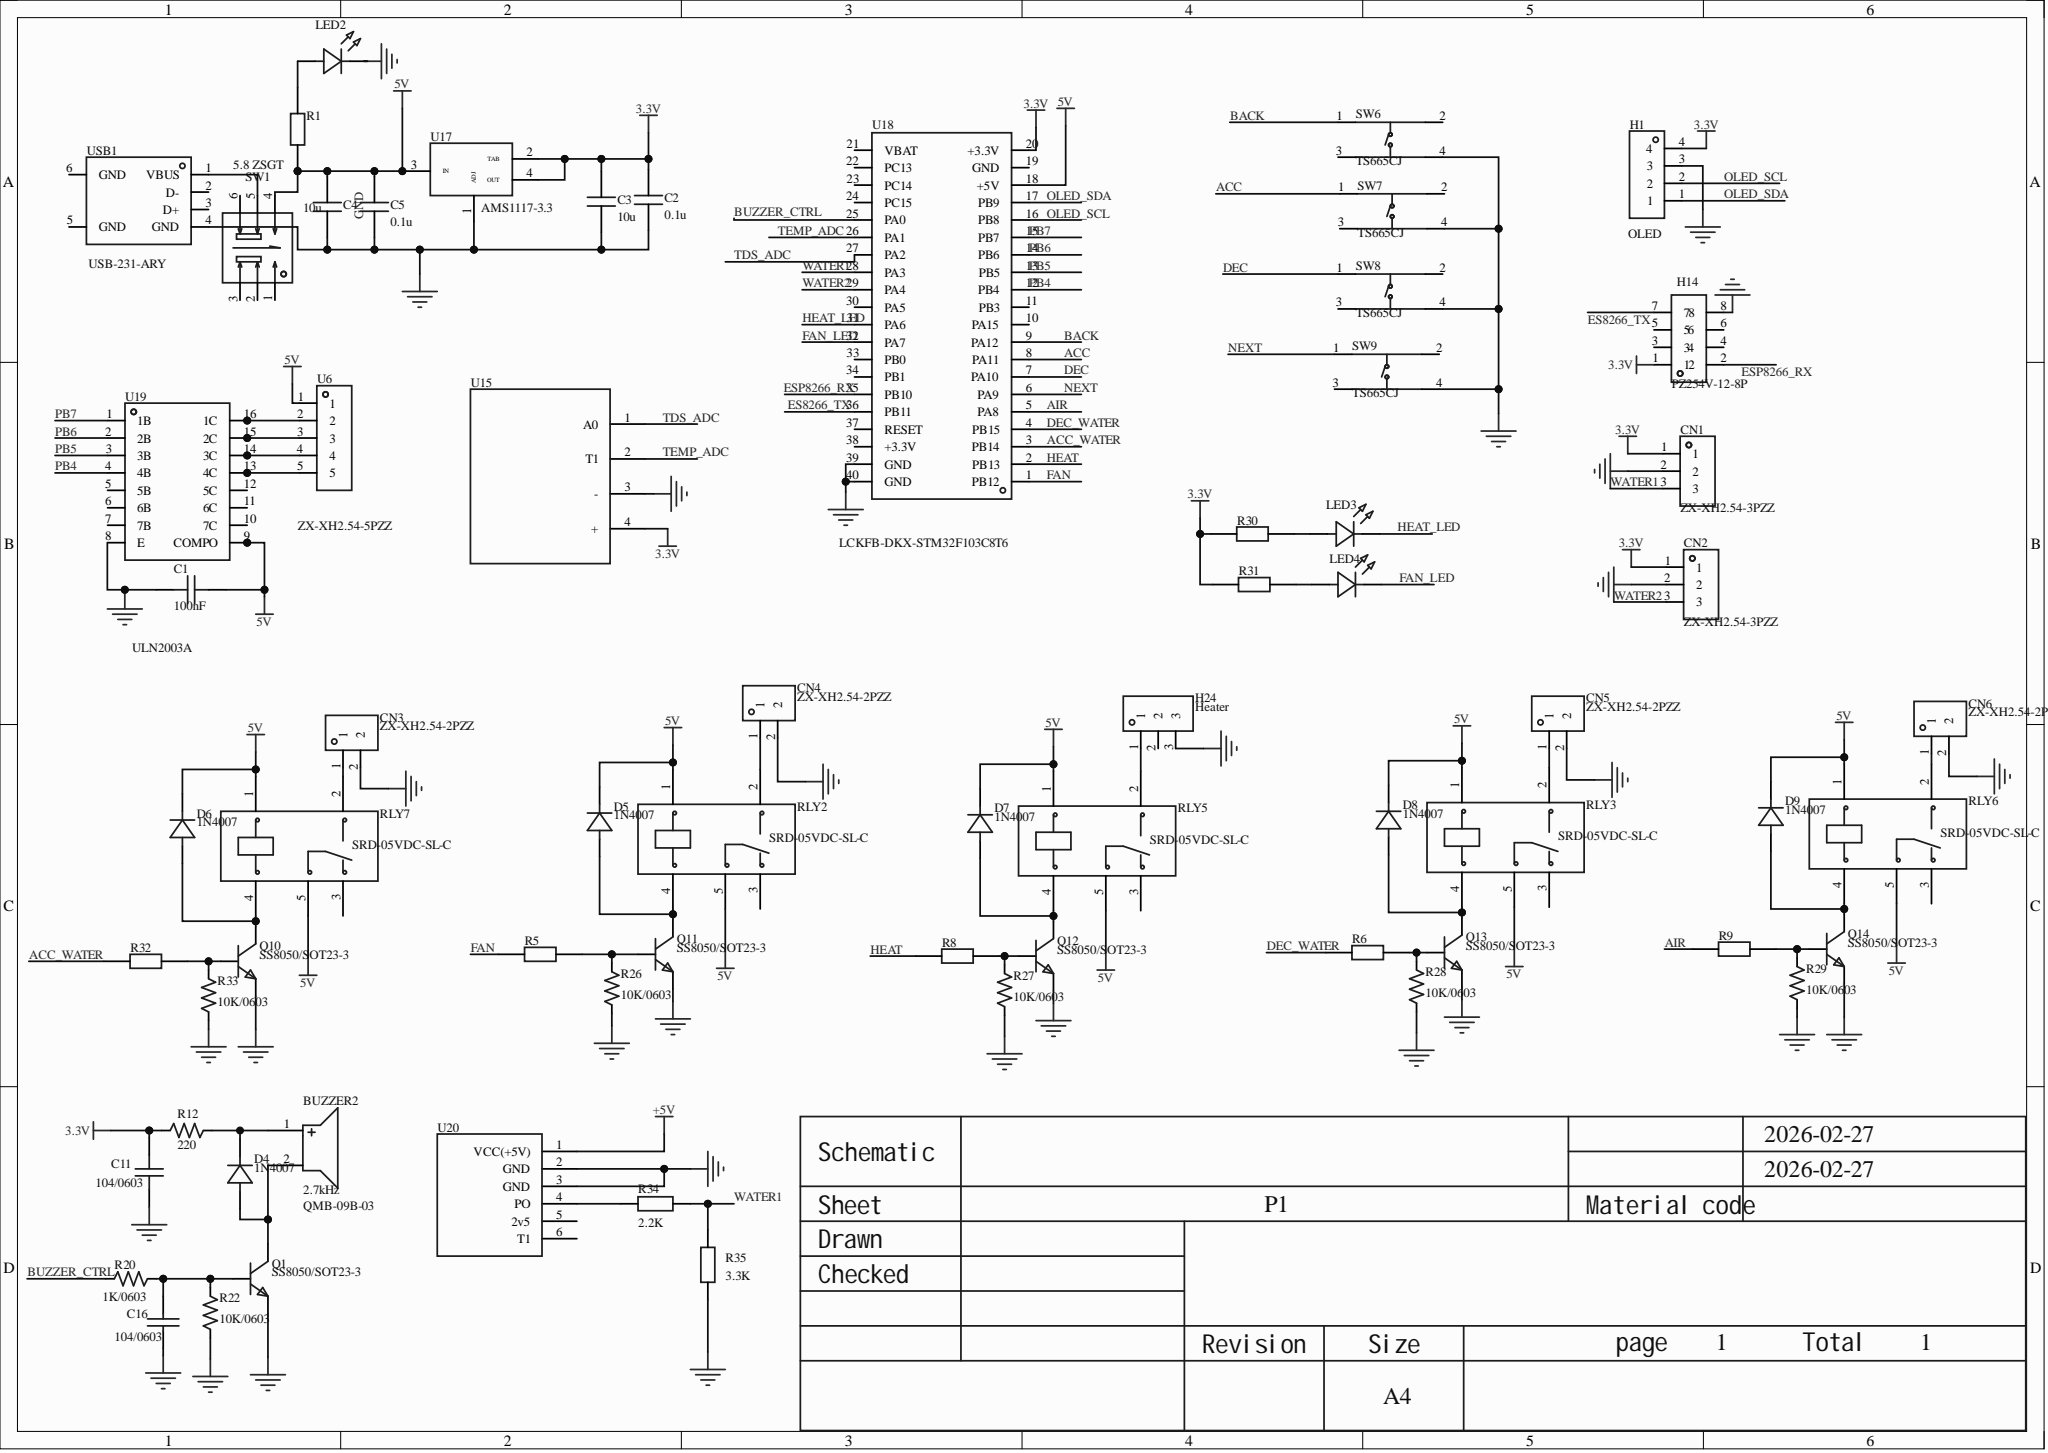Circuit board | Altium Designer | 67 parts | 50 nets
Bill of materials:
Comment,Description,Designator,Footprint,LibRef,Quantity
"2.7kHz","Drive:Passive (external drive);Construction:Electromagnetic;Frequency:2.7kHz;Sound pressure (SPL):85dB;","BUZZER2","BUZ-TH_BD9.0-P4.00-D0.6-FD","QMB-09B-03","1"
"100nF","Capacitance:100nF;Tolerance:±20%;Rated voltage:50V;Temperature coefficient:Y5V;","C1","c0805","CC1H104MC1FD3F6C10MF","1"
"0.1u","","C2, C5","c0805","电容","2"
"10u","","C3, C4","c0805","电容","2"
"104/0603","Capacitance:47uF;Tolerance:±20%;Rated voltage:10V;Temperature coefficient:X5R;, [NoValue]","C11, C16","c0805","CGA0805X5R476M100MT, 1uF","2"
"ZX-XH2.54-3PZZ","Pin structure:1x3P;Pitch:2.5mm;Mounting:Through-hole;Reference series:XH;Total pins:3P;Rows:1;Pins per row:3;Row spacing:-;Rated current:3A;Contact material:Brass;Contact plating:Tin;Operating temperature:-25℃~+85℃;","CN1, CN2","CONN-TH_3P-P2.54_2501S-3P","ZX-XH2.54-3PZZ","2"
"ZX-XH2.54-2PZZ","Pin structure:1x2P;Pitch:2.5mm;Mounting:Through-hole;Reference series:XH;Total pins:2P;Rows:1;Pins per row:2;Row spacing:-;Rated current:3A;Contact material:Brass;Contact plating:Tin;Operating temperature:-25℃~+85℃;","CN3, CN4, CN5, CN6","CONN-TH_2P-P2.50_HX25003-2A","ZX-XH2.54-2PZZ","4"
"1N4007","Diode configuration:Independent;Forward voltage (Vf):1V@1A;DC reverse voltage (Vr):1kV;Rectified current:1A;","D4, D5, D6, D7, D8, D9","DO-41_BD2.4-L4.7-P8.70-D0.8-RD","1N4007_C2985028","6"
"OLED","Pin structure:1x4P;Pitch:2.54mm;Row spacing:-;Round/square pin:Square pin;Mounting type:Through-hole;Rows:Single row;Total pins:4P;Rated current:3A;Rated voltage:250V;Mating pin length:6mm;Housing height:2.5mm;Termination pin length:3mm;Contact material:-;Operating temperature range:-40℃~+105℃;Color:Black;","H1","oled","PZ254V-11-04P","1"
"PZ254V-12-8P","Pin structure:2x4P;Pitch:2.54mm;Row spacing:2.54mm;Round/square pin:Square pin;Mounting type:Through-hole;Rows:Dual row;Total pins:8P;Rated current:-;Rated voltage:-;Mating pin length:6mm;Housing height:2.5mm;Termination pin length:3mm;Contact material:Brass;Contact plating:-;Operating temperature range:-40℃~+105℃;Color:Black;","H14","ESP8266","PZ254V-12-8P","1"
"Heater","Pin structure:1x3P;Pitch:2.54mm;Row spacing:-;Round/square pin:Square pin;Mounting type:Through-hole;Rows:Single row;Total pins:3P;Rated current:3A;Rated voltage:250V;Mating pin length:6mm;Housing height:2.5mm;Termination pin length:3mm;Operating temperature range:-40℃~+105℃;Color:Black;","H24","HDR-TH_3P-P2.54-V-M","PZ254V-11-03P","1"
"L-7113SGC","","LED2, LED3, LED4","LED-TH_BD5.9-P2.54-FD","L-7113SGC","3"
"SS8050/SOT23-3","Transistor type:NPN;Collector current (Ic):1.5A;Collector-emitter breakdown voltage (Vceo):25V;Power (Pd):300mW;DC current gain (hFE@Ic,Vce):200@800mA,1V;","Q1, Q10, Q11, Q12, Q13, Q14","SOT-23-3_L2.9-W1.3-P1.90-LS2.4-BR","SS8050(RANGE:200-350)_C2150","6"
"","","R1, R5, R6, R8, R9, R30, R31, R32","c0805","电阻","8"
"220","","R12","c0805","560","1"
"1K/0603","","R20","c0805","560","1"
"10K/0603","","R22, R26, R27, R28, R29, R33","c0805","560","6"
"2.2K","","R34","R0603","Res_0603","1"
"3.3K","","R35","R0603","Res_0603","1"
"SRD-05VDC-SL-C","Coil voltage:5V;Contact form:1C (SPDT);Contact rating (resistive):-;Max switching voltage:250V@AC;Max switching current:15A;","RLY2, RLY3, RLY5, RLY6, RLY7","RELAY-TH_SRD-XXVDC-XL-C","SRD-05VDC-SL-C","5"
"5.8 ZSGT","Circuit:DPDT;Self-lock/no-lock:Self-lock;Mounting:Through-hole;Contact current:110mA;Rated voltage (DC):30V;With lamp:Without;Actuation force:1.5N;Mechanical life:10万 cycles;","SW1","SW-TH_5.8ZSGT","5.8 ZSGT","1"
"TS665CJ","Circuit:SPST;Button shape:Round button;Mounting:Through-hole;Switch length:6mm;Switch width:6mm;Switch height:5mm;Contact current:50mA;Rated voltage (DC):12V;With lamp:-;Mechanical life:-;","SW6, SW7, SW8, SW9","SW-TH_4P-L6.0-W6.0-P4.50-LS6.5","TS665CJ","4"
"ZX-XH2.54-5PZZ","Pin structure:1x5P;Pitch:2.5mm;Mounting:Through-hole;Reference series:XH;Total pins:5P;Rows:1;Pins per row:5;Row spacing:-;Rated current:3A;Contact material:Brass;Contact plating:Tin;Operating temperature range:-25℃~+85℃;","U6","CONN-TH_5P-P2.50_ZX-XH2.54-5PZZ","ZX-XH2.54-5PZZ","1"
"","","U15","TDS模块","TDS模块","1"
"AMS1117-3.3","","U17","sot-223","AMS1117-3.3","1"
"LCKFB-DKX-STM32F103C8T6","","U18","CONN-TH_L53.3-W22.9_STM32F103C8T6-CARD","LCKFB-DKX-STM32F103C8T6","1"
"ULN2003A","Channels:Seven;Collector-emitter breakdown voltage (Vceo):50V;","U19","SOP-16_L10.0-W3.9-P1.27-LS6.0-BL","ULN2003A_C482013","1"
"","pH sensor module, analog output PO pin","U20","HDR-M-2.54_1X6","PH-4502C","1"
"USB-231-ARY","Connector type:Type-A;Protocol standard:USB 2.0;Gender:Female;Mounting:Right-angle;Contact count:4P;Port count:1;Rated current - power:1.5A;Operating temperature:-20℃~+70℃;","USB1","USB-A-TH_USB-231-ARY","USB-231-ARY","1"
Netlist (Protel format):
[
BUZZER2
BUZ-TH_BD9.0-P4.00-D0.6-FD
2.7kHz



]
[
C1
c0805
100nF



]
[
C2
c0805
0.1u



]
[
C3
c0805
10u



]
[
C4
c0805
10u



]
[
C5
c0805
0.1u



]
[
C11
c0805
104/0603



]
[
C16
c0805
104/0603



]
[
CN1
CONN-TH_3P-P2.54_2501S-3P
ZX-XH2.54-3PZZ



]
[
CN2
CONN-TH_3P-P2.54_2501S-3P
ZX-XH2.54-3PZZ



]
[
CN3
CONN-TH_2P-P2.50_HX25003-2A
ZX-XH2.54-2PZZ



]
[
CN4
CONN-TH_2P-P2.50_HX25003-2A
ZX-XH2.54-2PZZ



]
[
CN5
CONN-TH_2P-P2.50_HX25003-2A
ZX-XH2.54-2PZZ



]
[
CN6
CONN-TH_2P-P2.50_HX25003-2A
ZX-XH2.54-2PZZ



]
[
D4
DO-41_BD2.4-L4.7-P8.70-D0.8-RD
1N4007



]
[
D5
DO-41_BD2.4-L4.7-P8.70-D0.8-RD
1N4007



]
[
D6
DO-41_BD2.4-L4.7-P8.70-D0.8-RD
1N4007



]
[
D7
DO-41_BD2.4-L4.7-P8.70-D0.8-RD
1N4007



]
[
D8
DO-41_BD2.4-L4.7-P8.70-D0.8-RD
1N4007



]
[
D9
DO-41_BD2.4-L4.7-P8.70-D0.8-RD
1N4007



]
[
H1
oled
OLED



]
[
H14
ESP8266
PZ254V-12-8P



]
[
H24
HDR-TH_3P-P2.54-V-M
Heater



]
[
LED2
LED-TH_BD5.9-P2.54-FD
L-7113SGC



]
[
LED3
LED-TH_BD5.9-P2.54-FD
L-7113SGC



]
[
LED4
LED-TH_BD5.9-P2.54-FD
L-7113SGC



]
[
Q1
SOT-23-3_L2.9-W1.3-P1.90-LS2.4-BR
SS8050/SOT23-3



]
[
Q10
SOT-23-3_L2.9-W1.3-P1.90-LS2.4-BR
SS8050/SOT23-3



]
[
Q11
SOT-23-3_L2.9-W1.3-P1.90-LS2.4-BR
SS8050/SOT23-3



]
[
Q12
SOT-23-3_L2.9-W1.3-P1.90-LS2.4-BR
SS8050/SOT23-3



]
[
Q13
SOT-23-3_L2.9-W1.3-P1.90-LS2.4-BR
SS8050/SOT23-3



]
[
Q14
SOT-23-3_L2.9-W1.3-P1.90-LS2.4-BR
SS8050/SOT23-3



]
[
R1
c0805




]
[
R5
c0805




]
[
R6
c0805




]
[
R8
c0805




]
[
R9
c0805




]
[
R12
c0805
220



]
[
R20
c0805
1K/0603



]
[
R22
c0805
10K/0603



]
[
R26
c0805
10K/0603



]
[
R27
c0805
10K/0603



]
[
R28
c0805
10K/0603



]
[
R29
c0805
10K/0603



]
[
R30
c0805




]
[
R31
c0805




]
[
R32
c0805




]
[
R33
c0805
10K/0603



]
[
R34
R0603
2.2K



]
[
R35
R0603
3.3K



]
[
RLY2
RELAY-TH_SRD-XXVDC-XL-C
SRD-05VDC-SL-C



]
[
RLY3
RELAY-TH_SRD-XXVDC-XL-C
SRD-05VDC-SL-C



]
[
RLY5
RELAY-TH_SRD-XXVDC-XL-C
SRD-05VDC-SL-C



]
[
RLY6
RELAY-TH_SRD-XXVDC-XL-C
SRD-05VDC-SL-C



]
[
RLY7
RELAY-TH_SRD-XXVDC-XL-C
SRD-05VDC-SL-C



]
[
SW1
SW-TH_5.8ZSGT
5.8 ZSGT



]
[
SW6
SW-TH_4P-L6.0-W6.0-P4.50-LS6.5
TS665CJ



]
[
SW7
SW-TH_4P-L6.0-W6.0-P4.50-LS6.5
TS665CJ



]
[
SW8
SW-TH_4P-L6.0-W6.0-P4.50-LS6.5
TS665CJ



]
[
SW9
SW-TH_4P-L6.0-W6.0-P4.50-LS6.5
TS665CJ



]
[
U6
CONN-TH_5P-P2.50_ZX-XH2.54-5PZZ
ZX-XH2.54-5PZZ



]
[
U15
TDS模块




]
[
U17
sot-223
AMS1117-3.3



]
[
U18
CONN-TH_L53.3-W22.9_STM32F103C8T6-CARD
LCKFB-DKX-STM32F103C8T6



]
[
U19
SOP-16_L10.0-W3.9-P1.27-LS6.0-BL
ULN2003A



]
[
U20
HDR-M-2.54_1X6




]
[
USB1
USB-A-TH_USB-231-ARY
USB-231-ARY



]
(
WATER2
CN2-3
U18-29
)
(
WATER1
CN1-3
R34-2
R35-2
U18-28
)
(
TEMP_ADC
U15-2
U18-26
)
(
TDS_ADC
U15-1
U18-27
)
(
OLED_SDA
H1-1
U18-17
)
(
OLED_SCL
H1-2
U18-16
)
(
NEXT
SW9-1
U18-6
)
(
NetU6_5
U6-5
U19-13
)
(
NetU6_4
U6-4
U19-14
)
(
NetU6_3
U6-3
U19-15
)
(
NetU6_2
U6-2
U19-16
)
(
NetSW1_5
SW1-5
USB1-1
)
(
NetR34_1
R34-1
U20-4
)
(
NetQ14_1
Q14-1
R9-2
R29-2
)
(
NetQ13_1
Q13-1
R6-2
R28-2
)
(
NetQ12_1
Q12-1
R8-2
R27-2
)
(
NetQ11_1
Q11-1
R5-2
R26-2
)
(
NetQ10_1
Q10-1
R32-2
R33-2
)
(
NetLED4_1
LED4-1
R31-1
)
(
NetLED3_1
LED3-1
R30-1
)
(
NetLED2_1
LED2-1
R1-2
)
(
NetH24_1
H24-1
RLY5-2
)
(
NetD9_2
D9-2
Q14-3
RLY6-4
)
(
NetD8_2
D8-2
Q13-3
RLY3-4
)
(
NetD7_2
D7-2
Q12-3
RLY5-4
)
(
NetD6_2
D6-2
Q10-3
RLY7-4
)
(
NetD5_2
D5-2
Q11-3
RLY2-4
)
(
NetCN6_1
CN6-1
RLY6-2
)
(
NetCN5_1
CN5-1
RLY3-2
)
(
NetCN4_1
CN4-1
RLY2-2
)
(
NetCN3_1
CN3-1
RLY7-2
)
(
NetC16_2
C16-2
Q1-1
R20-2
R22-2
)
(
NetBUZZER2_2
BUZZER2-2
D4-2
Q1-3
)
(
NetBUZZER2_1
BUZZER2-1
D4-1
R12-2
)
(
HEAT_LED
LED3-2
U18-31
)
(
HEAT
R8-1
U18-2
)
(
GND
C1-1
C2-1
C3-1
C4-1
C5-1
C11-1
C16-1
CN1-2
CN2-2
CN3-2
CN4-2
CN5-2
CN6-2
H1-3
H14-8
H24-3
LED2-2
Q1-2
Q10-2
Q11-2
Q12-2
Q13-2
Q14-2
R22-1
R26-1
R27-1
R28-1
R29-1
R33-1
R35-1
SW6-4
SW7-4
SW8-4
SW9-4
U15-3
U17-1
U18-39
U18-40
U20-2
U20-3
USB1-4
)
(
FAN_LED
LED4-2
U18-32
)
(
FAN
R5-1
U18-1
)
(
ESP8266_RX
H14-2
U18-35
)
(
ES8266_TX
H14-7
U18-36
)
(
DEC_WATER
R6-1
U18-4
)
(
DEC
SW8-1
U18-7
)
(
BUZZER_CTRL
R20-1
U18-25
)
(
BACK
SW6-1
U18-9
)
(
AIR
R9-1
U18-5
)
(
ACC_WATER
R32-1
U18-3
)
(
ACC
SW7-1
U18-8
)
(
5V
C1-2
C4-2
C5-2
D5-1
D6-1
D7-1
D8-1
D9-1
R1-1
RLY2-1
RLY2-5
RLY3-1
RLY3-5
RLY5-1
RLY5-5
RLY6-1
RLY6-5
RLY7-1
RLY7-5
SW1-4
U6-1
U17-3
U18-18
U19-9
)
(
3.3V
C2-2
C3-2
C11-2
CN1-1
CN2-1
H1-4
H14-1
R12-1
R30-2
R31-2
U15-4
U17-2
U17-4
U18-20
)